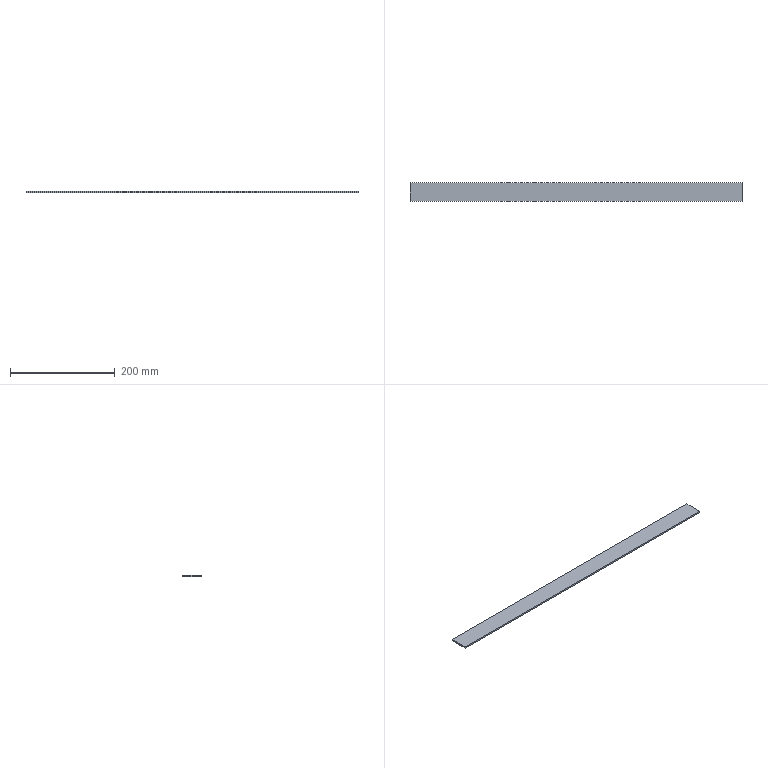Part | SolidWorks | features Extrusion 1 | 1 solid | 6 faces | box 634 x 35 x 3 mm | volume 66570 mm3 | plane 6
STEP:
#1=CARTESIAN_POINT('',(317.,-17.5,0.));
#2=VERTEX_POINT('',#1);
#3=CARTESIAN_POINT('',(317.,17.5,0.));
#4=VERTEX_POINT('',#3);
#5=CARTESIAN_POINT('',(317.,17.5,0.));
#6=DIRECTION('',(0.,1.,0.));
#7=VECTOR('',#6,1000.);
#8=LINE('',#5,#7);
#9=EDGE_CURVE('',#2,#4,#8,.T.);
#10=ORIENTED_EDGE('',*,*,#9,.T.);
#11=CARTESIAN_POINT('',(317.,17.5,3.));
#12=VERTEX_POINT('',#11);
#13=CARTESIAN_POINT('',(317.,17.5,3.));
#14=DIRECTION('',(0.,0.,-1.));
#15=VECTOR('',#14,1000.);
#16=LINE('',#13,#15);
#17=EDGE_CURVE('',#12,#4,#16,.T.);
#18=ORIENTED_EDGE('',*,*,#17,.F.);
#19=CARTESIAN_POINT('',(317.,-17.5,3.));
#20=VERTEX_POINT('',#19);
#21=CARTESIAN_POINT('',(317.,17.5,3.));
#22=DIRECTION('',(0.,1.,0.));
#23=VECTOR('',#22,1000.);
#24=LINE('',#21,#23);
#25=EDGE_CURVE('',#20,#12,#24,.T.);
#26=ORIENTED_EDGE('',*,*,#25,.F.);
#27=CARTESIAN_POINT('',(317.,-17.5,3.));
#28=DIRECTION('',(0.,0.,-1.));
#29=VECTOR('',#28,1000.);
#30=LINE('',#27,#29);
#31=EDGE_CURVE('',#20,#2,#30,.T.);
#32=ORIENTED_EDGE('',*,*,#31,.T.);
#33=EDGE_LOOP('',(#10,#18,#26,#32));
#34=FACE_OUTER_BOUND('',#33,.T.);
#35=CARTESIAN_POINT('',(317.,17.5,3.));
#36=DIRECTION('',(-1.,0.,0.));
#37=DIRECTION('',(0.,0.,1.));
#38=AXIS2_PLACEMENT_3D('',#35,#36,#37);
#39=PLANE('',#38);
#40=ADVANCED_FACE('',(#34),#39,.F.);
#41=CARTESIAN_POINT('',(-317.,17.5,0.));
#42=VERTEX_POINT('',#41);
#43=CARTESIAN_POINT('',(-317.,17.5,0.));
#44=DIRECTION('',(-1.,0.,0.));
#45=VECTOR('',#44,1000.);
#46=LINE('',#43,#45);
#47=EDGE_CURVE('',#4,#42,#46,.T.);
#48=ORIENTED_EDGE('',*,*,#47,.T.);
#49=CARTESIAN_POINT('',(-317.,17.5,3.));
#50=VERTEX_POINT('',#49);
#51=CARTESIAN_POINT('',(-317.,17.5,3.));
#52=DIRECTION('',(0.,0.,-1.));
#53=VECTOR('',#52,1000.);
#54=LINE('',#51,#53);
#55=EDGE_CURVE('',#50,#42,#54,.T.);
#56=ORIENTED_EDGE('',*,*,#55,.F.);
#57=CARTESIAN_POINT('',(-317.,17.5,3.));
#58=DIRECTION('',(-1.,0.,0.));
#59=VECTOR('',#58,1000.);
#60=LINE('',#57,#59);
#61=EDGE_CURVE('',#12,#50,#60,.T.);
#62=ORIENTED_EDGE('',*,*,#61,.F.);
#63=ORIENTED_EDGE('',*,*,#17,.T.);
#64=EDGE_LOOP('',(#48,#56,#62,#63));
#65=FACE_OUTER_BOUND('',#64,.T.);
#66=CARTESIAN_POINT('',(-317.,17.5,3.));
#67=DIRECTION('',(0.,-1.,0.));
#68=DIRECTION('',(0.,0.,-1.));
#69=AXIS2_PLACEMENT_3D('',#66,#67,#68);
#70=PLANE('',#69);
#71=ADVANCED_FACE('',(#65),#70,.F.);
#72=CARTESIAN_POINT('',(-317.,-17.5,0.));
#73=VERTEX_POINT('',#72);
#74=CARTESIAN_POINT('',(-317.,17.5,0.));
#75=DIRECTION('',(0.,-1.,0.));
#76=VECTOR('',#75,1000.);
#77=LINE('',#74,#76);
#78=EDGE_CURVE('',#42,#73,#77,.T.);
#79=ORIENTED_EDGE('',*,*,#78,.T.);
#80=CARTESIAN_POINT('',(-317.,-17.5,3.));
#81=VERTEX_POINT('',#80);
#82=CARTESIAN_POINT('',(-317.,-17.5,3.));
#83=DIRECTION('',(0.,0.,-1.));
#84=VECTOR('',#83,1000.);
#85=LINE('',#82,#84);
#86=EDGE_CURVE('',#81,#73,#85,.T.);
#87=ORIENTED_EDGE('',*,*,#86,.F.);
#88=CARTESIAN_POINT('',(-317.,17.5,3.));
#89=DIRECTION('',(0.,-1.,0.));
#90=VECTOR('',#89,1000.);
#91=LINE('',#88,#90);
#92=EDGE_CURVE('',#50,#81,#91,.T.);
#93=ORIENTED_EDGE('',*,*,#92,.F.);
#94=ORIENTED_EDGE('',*,*,#55,.T.);
#95=EDGE_LOOP('',(#79,#87,#93,#94));
#96=FACE_OUTER_BOUND('',#95,.T.);
#97=CARTESIAN_POINT('',(-317.,17.5,3.));
#98=DIRECTION('',(1.,0.,0.));
#99=DIRECTION('',(0.,0.,-1.));
#100=AXIS2_PLACEMENT_3D('',#97,#98,#99);
#101=PLANE('',#100);
#102=ADVANCED_FACE('',(#96),#101,.F.);
#103=CARTESIAN_POINT('',(-317.,-17.5,0.));
#104=DIRECTION('',(1.,0.,0.));
#105=VECTOR('',#104,1000.);
#106=LINE('',#103,#105);
#107=EDGE_CURVE('',#73,#2,#106,.T.);
#108=ORIENTED_EDGE('',*,*,#107,.T.);
#109=ORIENTED_EDGE('',*,*,#31,.F.);
#110=CARTESIAN_POINT('',(-317.,-17.5,3.));
#111=DIRECTION('',(1.,0.,0.));
#112=VECTOR('',#111,1000.);
#113=LINE('',#110,#112);
#114=EDGE_CURVE('',#81,#20,#113,.T.);
#115=ORIENTED_EDGE('',*,*,#114,.F.);
#116=ORIENTED_EDGE('',*,*,#86,.T.);
#117=EDGE_LOOP('',(#108,#109,#115,#116));
#118=FACE_OUTER_BOUND('',#117,.T.);
#119=CARTESIAN_POINT('',(-317.,-17.5,3.));
#120=DIRECTION('',(0.,1.,0.));
#121=DIRECTION('',(0.,0.,1.));
#122=AXIS2_PLACEMENT_3D('',#119,#120,#121);
#123=PLANE('',#122);
#124=ADVANCED_FACE('',(#118),#123,.F.);
#125=ORIENTED_EDGE('',*,*,#25,.T.);
#126=ORIENTED_EDGE('',*,*,#61,.T.);
#127=ORIENTED_EDGE('',*,*,#92,.T.);
#128=ORIENTED_EDGE('',*,*,#114,.T.);
#129=EDGE_LOOP('',(#125,#126,#127,#128));
#130=FACE_OUTER_BOUND('',#129,.T.);
#131=CARTESIAN_POINT('',(0.,0.,3.));
#132=DIRECTION('',(0.,0.,1.));
#133=DIRECTION('',(1.,0.,0.));
#134=AXIS2_PLACEMENT_3D('',#131,#132,#133);
#135=PLANE('',#134);
#136=ADVANCED_FACE('',(#130),#135,.T.);
#137=ORIENTED_EDGE('',*,*,#9,.F.);
#138=ORIENTED_EDGE('',*,*,#107,.F.);
#139=ORIENTED_EDGE('',*,*,#78,.F.);
#140=ORIENTED_EDGE('',*,*,#47,.F.);
#141=EDGE_LOOP('',(#137,#138,#139,#140));
#142=FACE_OUTER_BOUND('',#141,.T.);
#143=CARTESIAN_POINT('',(0.,0.,0.));
#144=DIRECTION('',(0.,0.,1.));
#145=DIRECTION('',(1.,0.,0.));
#146=AXIS2_PLACEMENT_3D('',#143,#144,#145);
#147=PLANE('',#146);
#148=ADVANCED_FACE('',(#142),#147,.F.);
#149=CLOSED_SHELL('',(#40,#71,#102,#124,#136,#148));
#150=MANIFOLD_SOLID_BREP('',#149);
#151=CARTESIAN_POINT('',(0.,0.,0.));
#152=DIRECTION('',(0.,0.,1.));
#153=DIRECTION('',(1.,0.,0.));
#154=AXIS2_PLACEMENT_3D('',#151,#152,#153);
#155=(LENGTH_UNIT()NAMED_UNIT(*)SI_UNIT(.MILLI.,.METRE.));
#156=UNCERTAINTY_MEASURE_WITH_UNIT(LENGTH_MEASURE(0.00001),#155,'','');
#157=(NAMED_UNIT(*)PLANE_ANGLE_UNIT()SI_UNIT($,.RADIAN.));
#158=(NAMED_UNIT(*)SI_UNIT($,.STERADIAN.)SOLID_ANGLE_UNIT());
#159=(GEOMETRIC_REPRESENTATION_CONTEXT(3)GLOBAL_UNCERTAINTY_ASSIGNED_CONTEXT((#156))GLOBAL_UNIT_ASSIGNED_CONTEXT((#155,#157,#158))REPRESENTATION_CONTEXT('',''));
#160=ADVANCED_BREP_SHAPE_REPRESENTATION('',(#150,#154),#159);